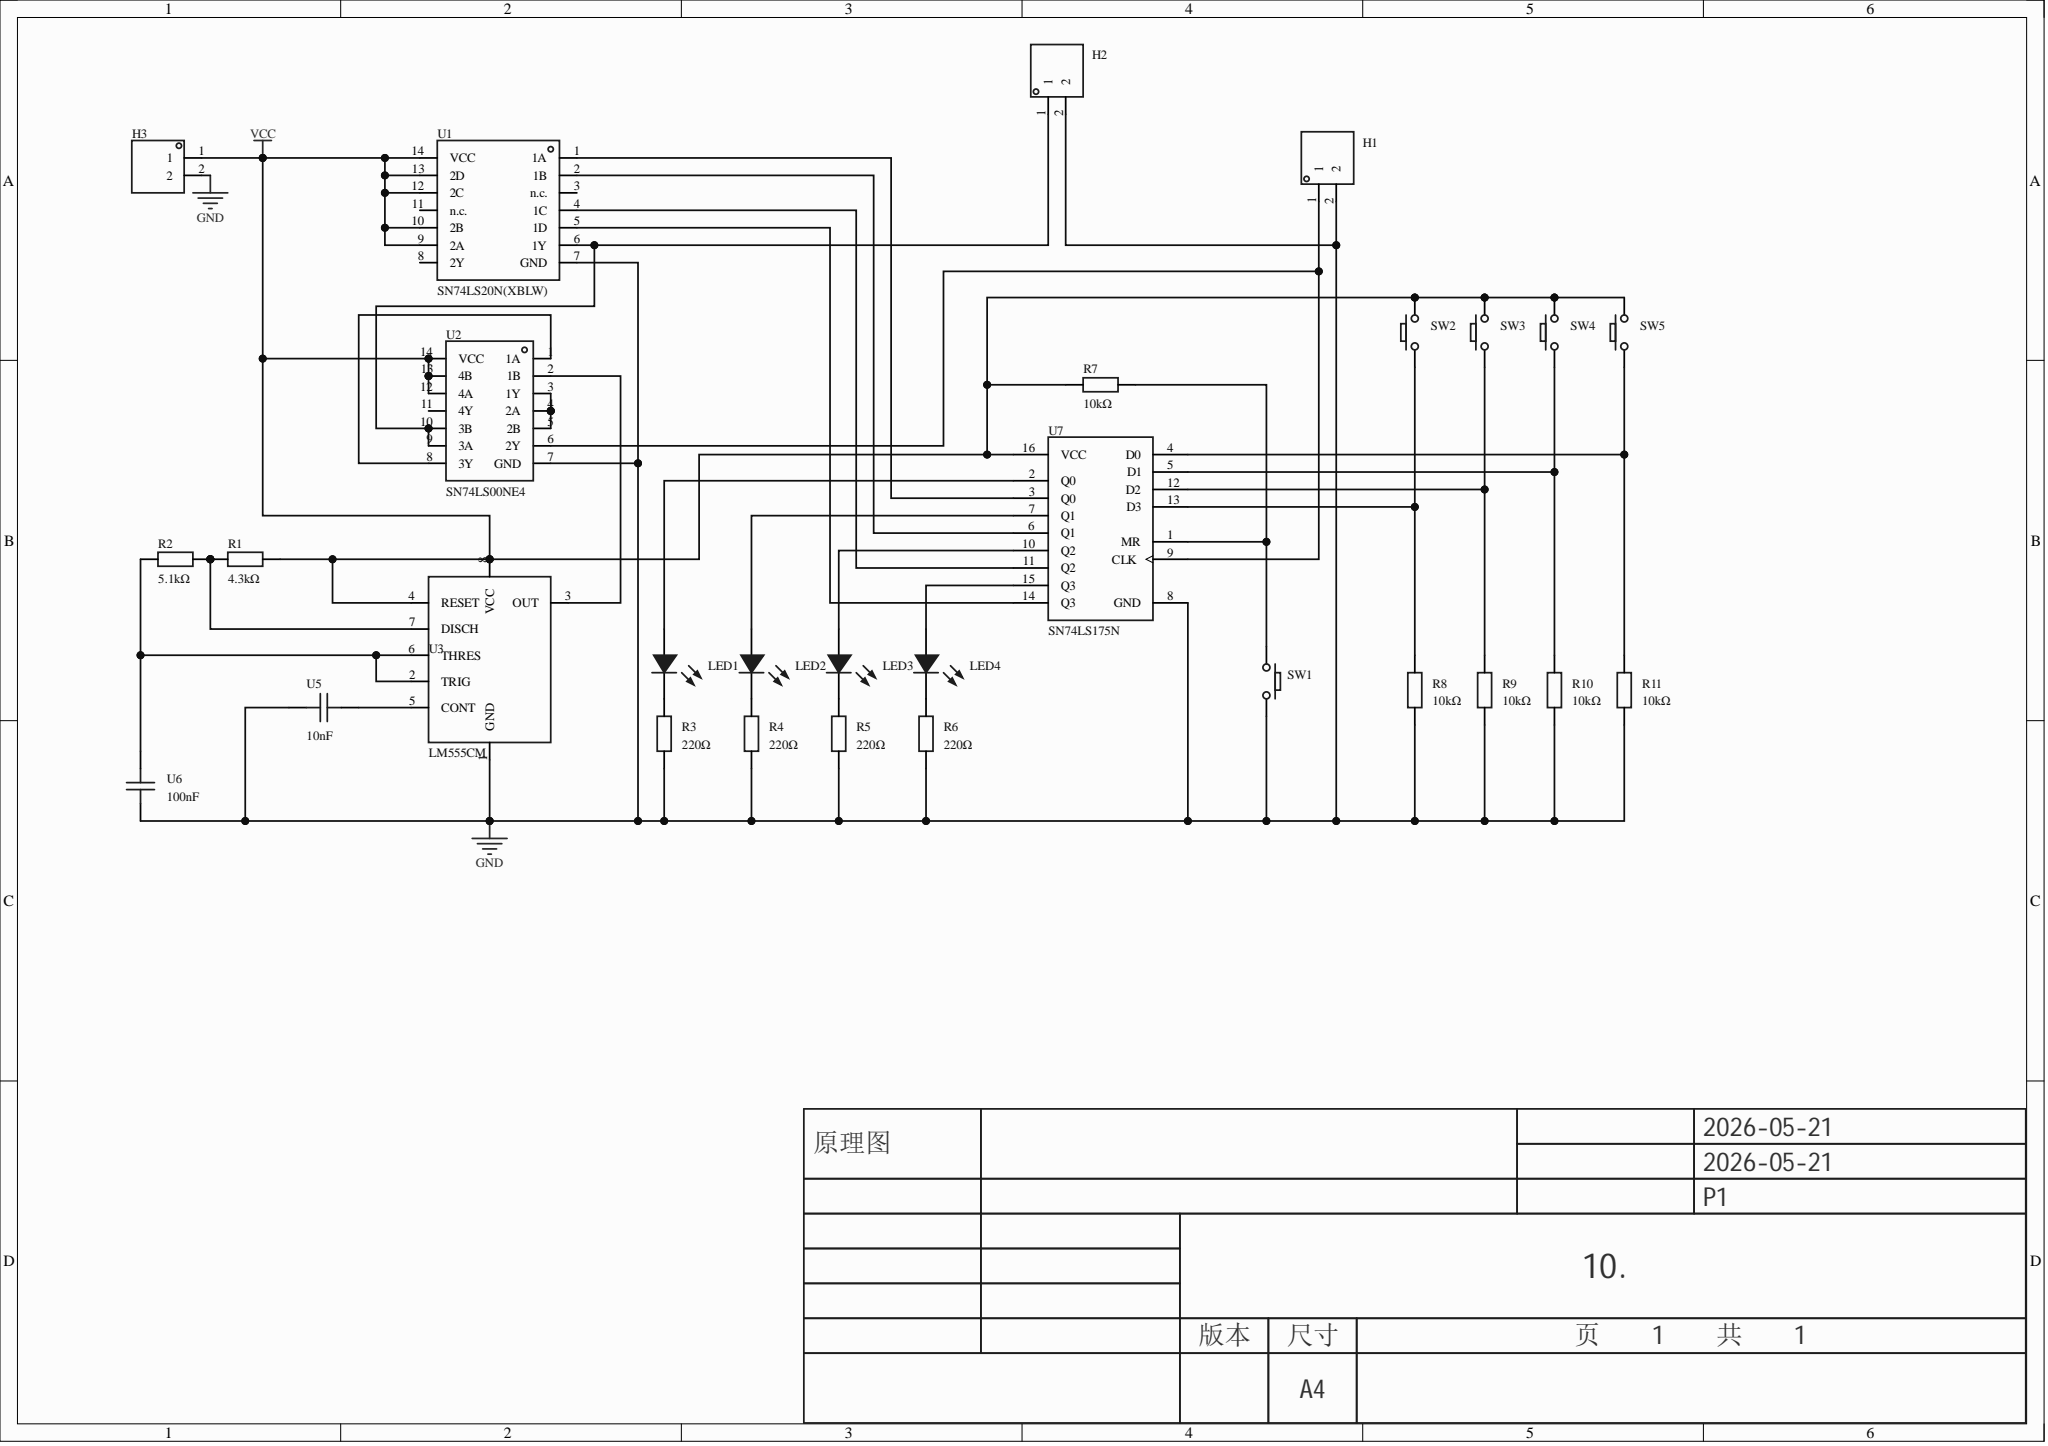Circuit board | Altium Designer | 29 parts | 27 nets
Bill of materials:
Comment,Description,Designator,Footprint,LibRef,Quantity
"","","H1, H2, H3","HDR-TH_2P-P2.54-V-M-1","HDR-M_2.54_1x2P","3"
"","","LED1, LED2, LED3, LED4","LED_TH-3mm","LED_TH-B_3mm","4"
"4.3kΩ","","R1","Res_1/8W","Res_AXIAL-1/8W","1"
"5.1kΩ","","R2","Res_1/8W","Res_AXIAL-1/8W","1"
"220Ω","","R3, R4, R5, R6","Res_1/8W","Res_AXIAL-1/8W","4"
"10kΩ","","R7, R8, R9, R10, R11","Res_1/8W","Res_AXIAL-1/8W","5"
"","","SW1, SW2, SW3, SW4, SW5","Key_TH_3.5x6x4.3","Key_TH_3.5x6x4.3","5"
"SN74LS20N(XBLW)","逻辑类型:与非门;通道数:2;工作电压:2V~6V;静态电流(Iq):2uA;传播延迟(tpd):18ns@4.5V；15ns@6V;","U1","DIP-14_L19.0-W6.4-P2.54-LS7.6-BL","SN74LS20N(XBLW)","1"
"SN74LS00NE4","SN74LS00 4 通道、双输入、4.75V 至 5.25V 双极与非门","U2","PDIP-14_L19.3-W6.4-P2.54-LS7.9-BL","SN74LS00NE4","1"
"LM555CM","NE555 单精度定时器","U3","PDIP-8_L9.6-W6.4-P2.54-LS7.9-BL-1","NE555PE4","1"
"10nF","","U5","CAP-TH_L5.0-W2.5-P5.00-D1.0","100nF","1"
"100nF","","U6","CAP-TH_L5.0-W2.5-P5.00-D1.0","100nF","1"
"SN74LS175N","","U7","DIP-16_L19.3-W6.4-P2.54-LS7.6-BL","SN74LS175N","1"
Netlist (Protel format):
[
H1
HDR-TH_2P-P2.54-V-M-1




]
[
H2
HDR-TH_2P-P2.54-V-M-1




]
[
H3
HDR-TH_2P-P2.54-V-M-1




]
[
LED1
LED_TH-3mm




]
[
LED2
LED_TH-3mm




]
[
LED3
LED_TH-3mm




]
[
LED4
LED_TH-3mm




]
[
R1
Res_1/8W
4.3kΩ



]
[
R2
Res_1/8W
5.1kΩ



]
[
R3
Res_1/8W
220Ω



]
[
R4
Res_1/8W
220Ω



]
[
R5
Res_1/8W
220Ω



]
[
R6
Res_1/8W
220Ω



]
[
R7
Res_1/8W
10kΩ



]
[
R8
Res_1/8W
10kΩ



]
[
R9
Res_1/8W
10kΩ



]
[
R10
Res_1/8W
10kΩ



]
[
R11
Res_1/8W
10kΩ



]
[
SW1
Key_TH_3.5x6x4.3




]
[
SW2
Key_TH_3.5x6x4.3




]
[
SW3
Key_TH_3.5x6x4.3




]
[
SW4
Key_TH_3.5x6x4.3




]
[
SW5
Key_TH_3.5x6x4.3




]
[
U1
DIP-14_L19.0-W6.4-P2.54-LS7.6-BL
SN74LS20N(XBLW)



]
[
U2
PDIP-14_L19.3-W6.4-P2.54-LS7.9-BL
SN74LS00NE4



]
[
U3
PDIP-8_L9.6-W6.4-P2.54-LS7.9-BL-1
LM555CM



]
[
U5
CAP-TH_L5.0-W2.5-P5.00-D1.0
10nF



]
[
U6
CAP-TH_L5.0-W2.5-P5.00-D1.0
100nF



]
[
U7
DIP-16_L19.3-W6.4-P2.54-LS7.6-BL
SN74LS175N



]
(
VCC
H3-1
R1-2
R7-1
SW2-B
SW3-B
SW4-B
SW5-B
U1-9
U1-10
U1-12
U1-13
U1-14
U2-12
U2-13
U2-14
U3-4
U3-8
U7-16
)
(
NetU3_5
U3-5
U5-1
)
(
NetU2_3
U2-3
U2-4
U2-5
)
(
NetU2_2
U2-2
U3-3
)
(
NetU2_1
U2-1
U2-8
)
(
NetU1_5
U1-5
U7-14
)
(
NetU1_4
U1-4
U7-11
)
(
NetU1_2
U1-2
U7-6
)
(
NetU1_1
U1-1
U7-3
)
(
NetR11_2
R11-2
SW5-A
U7-4
)
(
NetR10_2
R10-2
SW4-A
U7-5
)
(
NetR9_2
R9-2
SW3-A
U7-12
)
(
NetR8_2
R8-2
SW2-A
U7-13
)
(
NetR7_2
R7-2
SW1-B
U7-1
)
(
NetR2_1
R2-1
U3-2
U3-6
U6-1
)
(
NetR1_1
R1-1
R2-2
U3-7
)
(
NetLED4_2
LED4-2
R6-2
)
(
NetLED4_1
LED4-1
U7-15
)
(
NetLED3_2
LED3-2
R5-2
)
(
NetLED3_1
LED3-1
U7-10
)
(
NetLED2_2
LED2-2
R4-2
)
(
NetLED2_1
LED2-1
U7-7
)
(
NetLED1_2
LED1-2
R3-2
)
(
NetLED1_1
LED1-1
U7-2
)
(
NetH2_1
H2-1
U1-6
U2-9
U2-10
)
(
NetH1_1
H1-1
U2-6
U7-9
)
(
GND
H1-2
H2-2
H3-2
R3-1
R4-1
R5-1
R6-1
R8-1
R9-1
R10-1
R11-1
SW1-A
U1-7
U2-7
U3-1
U5-2
U6-2
U7-8
)